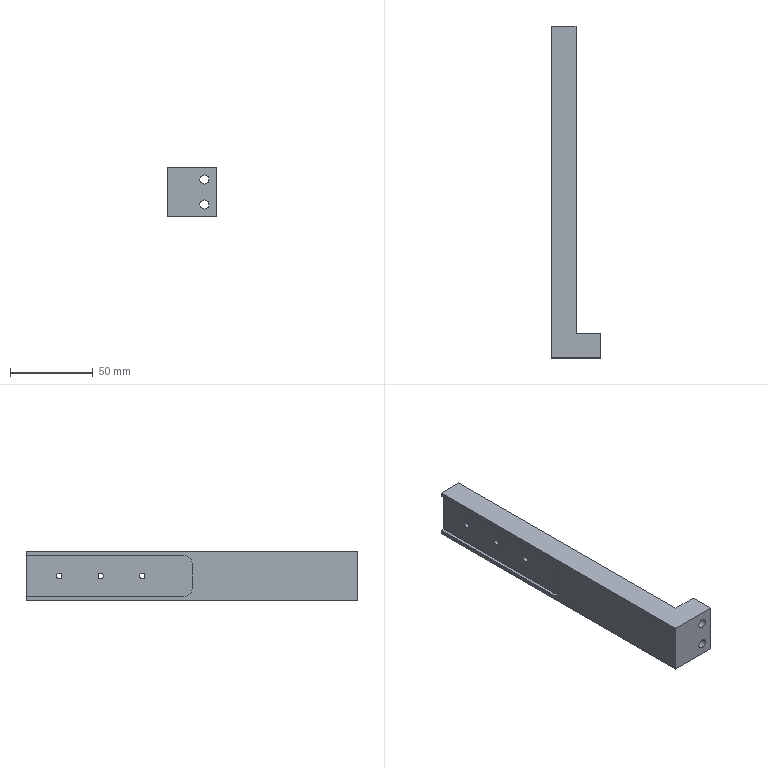CAM job | NX | 3+2 milling, drilling | part box 30 x 200 x 30 mm | stock box 35 x 205 x 35 mm
Tools:
number,name,description,diameter,corner_radius,flute_length,length,flutes
9,D10,平底铣刀-粗,10.0,0.0,35.0,75.0,2
7,D6-J,平底铣刀-精,6.0,0.0,25.0,75.0,2
10,D10-J,平底铣刀-精,10.0,0.0,35.0,75.0,2
1,D80R0.8_FLYCUTTER,圆鼻刀-粗,80.0,0.8,50.0,75.0,2
1,D80R0.8_FLYCUTTER-J,圆鼻刀-精,80.0,0.8,50.0,75.0,2
2,D6_CHAMFER,倒角刀,6.0,0.0,3.0,25.0,2
21,M4X0.7,丝锥,3.3,0.0,35.0,50.0,2
13,ZT3.4,钻头,3.4,0.0,35.0,50.0,2
Operations:
program,operation,operation_type,tool,method,geometry_group,spindle_rpm,surface_speed,feed_per_tooth,feed_cut,feed_plunge,cut_length_mm,path_length_mm,cut_time_min,machine_time_min
B,FLOORWALL_FACE1PASSROUGH_COPY,VolumeBased25DMillingOperation,D80R0.8_FLYCUTTER,LAYER_ROUGH-DEPTHK-STEPG,W-B,2800.0,703.696,0.5357,3000.0,100.0,2773.746,5765.966,0.9246,1.224
B,FLOORWALL_FACEFINISH_COPY,VolumeBased25DMillingOperation,D80R0.8_FLYCUTTER-J,SIDEFINISH-DEPTHK-STEPG,W-B,4000.0,1005.28,0.125,1000.0,100.0,307.998,403.998,0.308,0.3176
B,FLOORWALL_LAYERROUGH-MED_COPY,VolumeBased25DMillingOperation,D10,LAYER_ROUGH-DEPTHK-STEPG,W-B,8000.0,251.327,0.3125,5000.0,100.0,29122.704,33623.654,5.824,6.275
B,NG_DRILLCHAMFER_2,Operation,D6_CHAMFER,METHOD,W-B,8000.0,150.796,0.0625,1000.0,0.0,15.6,217.559,0.0156,0.0358
B,FLATDEBURR6X45L_COPY,SurfaceContour,D6_CHAMFER,STEEP_CHAMFER-DEPTH0-STEPG,W-B,6500.0,122.519,0.1154,1500.0,100.0,550.399,998.731,0.3669,0.4118
B,FLOORWALL_FINISHFLOOR-MED_COPY,VolumeBased25DMillingOperation,D10-J,FINISH_STEPDEPTHOFF,W-B,8000.0,251.32,0.0625,1000.0,100.0,1479.171,1535.171,1.479,1.485
B,FLOORWALL_FINISHSIDE-MED-SELFLOOR_COPY,VolumeBased25DMillingOperation,D10-J,SIDEFINISH-DEPTHK-STEPG,W-B,8000.0,251.32,0.0625,1000.0,100.0,48.682,105.682,0.0487,0.0544
A,TOPFACE,FaceMilling,D80R0.8_FLYCUTTER,SIDEFINISH-DEPTHK-STEPG,W-A,4500.0,1385.0,0.1667,1500.0,100.0,294.0,390.0,0.196,0.2056
A,PROFILEROUGH_2,VolumeBased25DMillingOperation,D10,METHOD,W-A,8000.0,251.327,0.375,6000.0,80.0,19683.294,19811.794,3.28,3.293
A,STEPROUGH_2,CavityMilling,D10,METHOD,W-A,9000.0,282.743,0.3333,6000.0,100.0,1971.924,2120.064,0.3287,0.3435
A,SPOT-DEPTH0.8,Operation,D6_CHAMFER,NONE,W-A,8000.0,150.796,0.0312,500.0,90.0,5.4,166.84,0.0108,0.0269
A,THRU-M4TAPDRILL,Operation,ZT3.4,NONE,W-A,3000.0,31.102,0.05,300.0,90.0,69.0,294.04,0.23,0.2525
A,BODYONLY,SurfaceContour,D6_CHAMFER,METHOD,W-A,8000.0,150.796,0.1875,3000.0,100.0,703.936,1002.005,0.2346,0.2645
A,NG_DRILLCHAMFER_1,Operation,D6_CHAMFER,METHOD,W-A,8000.0,150.796,0.0312,500.0,0.0,15.6,191.559,0.0312,0.0488
A,THRU-M4TAP,Operation,M4X0.7,METHOD,W-A,600.0,6.22,0.0006,0.7,90.0,51.0,258.04,72.857,72.878
A,BOTTOMFINISH_1,VolumeBased25DMillingOperation,D6-J,METHOD,W-A,9000.0,169.646,0.0833,1500.0,100.0,621.041,724.041,0.414,0.4243
A,BOTTOMSIDEFINISH_3,VolumeBased25DMillingOperation,D6-J,METHOD,W-A,9000.0,169.646,0.0556,1000.0,100.0,221.088,324.078,0.2211,0.2314
A,PROFILESEMI_2,VolumeBased25DMillingOperation,D10-J,METHOD,W-A,9000.0,169.646,0.0667,1200.0,100.0,1489.122,1911.151,1.241,1.283